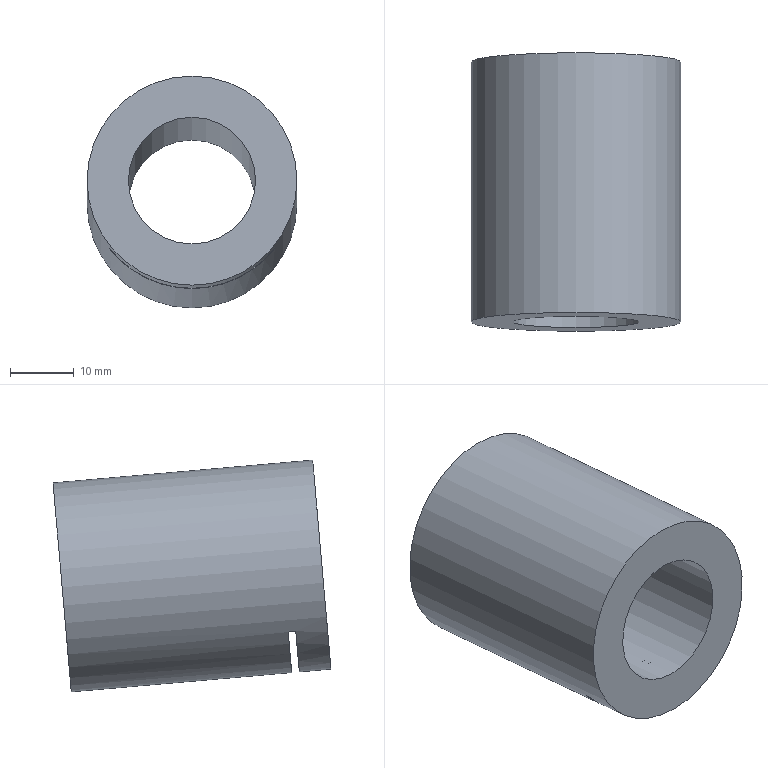Part | NX | features solid 2 | 1 solid | 7 faces | box 33 x 43.72 x 36.448 mm | volume 22047 mm3 | plane 5 | cylinder 2 | commonest cylinder face diameters 20 x1 33 x1
STEP:
#1=CARTESIAN_POINT('',(398.525,-75.036,-22.502));
#2=VERTEX_POINT('',#1);
#3=CARTESIAN_POINT('',(398.525,-76.474,-38.939));
#4=DIRECTION('',(0.,0.9962,-0.08716));
#5=DIRECTION('',(0.,0.08716,0.9962));
#6=AXIS2_PLACEMENT_3D('',#3,#4,#5);
#7=CIRCLE('',#6,16.5);
#8=EDGE_CURVE('',#2,#2,#7,.F.);
#9=ORIENTED_EDGE('',*,*,#8,.T.);
#10=EDGE_LOOP('',(#9));
#11=FACE_BOUND('',#10,.T.);
#12=CARTESIAN_POINT('',(398.525,-118.756,-51.803));
#13=VERTEX_POINT('',#12);
#14=CARTESIAN_POINT('',(398.525,-117.318,-35.366));
#15=DIRECTION('',(0.,-0.9962,0.08716));
#16=DIRECTION('',(0.,-0.08716,-0.9962));
#17=AXIS2_PLACEMENT_3D('',#14,#15,#16);
#18=CIRCLE('',#17,16.5);
#19=EDGE_CURVE('',#13,#13,#18,.T.);
#20=ORIENTED_EDGE('',*,*,#19,.F.);
#21=EDGE_LOOP('',(#20));
#22=FACE_BOUND('',#21,.T.);
#23=CARTESIAN_POINT('',(411.573,-113.217,-45.863));
#24=VERTEX_POINT('',#23);
#25=CARTESIAN_POINT('',(411.573,-112.021,-45.968));
#26=VERTEX_POINT('',#25);
#27=CARTESIAN_POINT('',(411.573,-76.358,-49.088));
#28=DIRECTION('',(0.,-0.9962,0.08716));
#29=VECTOR('',#28,1000.);
#30=LINE('',#27,#29);
#31=EDGE_CURVE('',#24,#26,#30,.F.);
#32=ORIENTED_EDGE('',*,*,#31,.T.);
#33=CARTESIAN_POINT('',(385.478,-112.021,-45.968));
#34=VERTEX_POINT('',#33);
#35=CARTESIAN_POINT('',(398.525,-111.141,-35.906));
#36=DIRECTION('',(0.,-0.9962,0.08716));
#37=DIRECTION('',(0.,-0.08716,-0.9962));
#38=AXIS2_PLACEMENT_3D('',#35,#36,#37);
#39=CIRCLE('',#38,16.5);
#40=EDGE_CURVE('',#26,#34,#39,.F.);
#41=ORIENTED_EDGE('',*,*,#40,.T.);
#42=CARTESIAN_POINT('',(385.478,-113.217,-45.863));
#43=VERTEX_POINT('',#42);
#44=CARTESIAN_POINT('',(385.478,-76.358,-49.088));
#45=DIRECTION('',(0.,-0.9962,0.08716));
#46=VECTOR('',#45,1000.);
#47=LINE('',#44,#46);
#48=EDGE_CURVE('',#34,#43,#47,.T.);
#49=ORIENTED_EDGE('',*,*,#48,.T.);
#50=CARTESIAN_POINT('',(398.525,-112.337,-35.802));
#51=DIRECTION('',(0.,-0.9962,0.08716));
#52=DIRECTION('',(0.,-0.08716,-0.9962));
#53=AXIS2_PLACEMENT_3D('',#50,#51,#52);
#54=CIRCLE('',#53,16.5);
#55=EDGE_CURVE('',#24,#43,#54,.F.);
#56=ORIENTED_EDGE('',*,*,#55,.F.);
#57=EDGE_LOOP('',(#32,#41,#49,#56));
#58=FACE_BOUND('',#57,.T.);
#59=CARTESIAN_POINT('',(398.525,-83.646,-38.312));
#60=DIRECTION('',(0.,-0.9962,0.08716));
#61=DIRECTION('',(0.,-0.08716,-0.9962));
#62=AXIS2_PLACEMENT_3D('',#59,#60,#61);
#63=CYLINDRICAL_SURFACE('',#62,16.5);
#64=ADVANCED_FACE('',(#11,#22,#58),#63,.T.);
#65=ORIENTED_EDGE('',*,*,#19,.T.);
#66=EDGE_LOOP('',(#65));
#67=FACE_BOUND('',#66,.T.);
#68=CARTESIAN_POINT('',(398.525,-118.189,-45.328));
#69=VERTEX_POINT('',#68);
#70=CARTESIAN_POINT('',(398.525,-117.318,-35.366));
#71=DIRECTION('',(0.,-0.9962,0.08716));
#72=DIRECTION('',(0.,-0.08716,-0.9962));
#73=AXIS2_PLACEMENT_3D('',#70,#71,#72);
#74=CIRCLE('',#73,10.);
#75=EDGE_CURVE('',#69,#69,#74,.T.);
#76=ORIENTED_EDGE('',*,*,#75,.F.);
#77=EDGE_LOOP('',(#76));
#78=FACE_BOUND('',#77,.T.);
#79=CARTESIAN_POINT('',(398.525,-117.318,-35.366));
#80=DIRECTION('',(0.,-0.9962,0.08716));
#81=DIRECTION('',(-1.,0.,0.));
#82=AXIS2_PLACEMENT_3D('',#79,#80,#81);
#83=PLANE('',#82);
#84=ADVANCED_FACE('',(#67,#78),#83,.T.);
#85=ORIENTED_EDGE('',*,*,#75,.T.);
#86=EDGE_LOOP('',(#85));
#87=FACE_BOUND('',#86,.T.);
#88=CARTESIAN_POINT('',(398.525,-75.602,-28.977));
#89=VERTEX_POINT('',#88);
#90=CARTESIAN_POINT('',(398.525,-76.474,-38.939));
#91=DIRECTION('',(0.,0.9962,-0.08716));
#92=DIRECTION('',(0.,0.08716,0.9962));
#93=AXIS2_PLACEMENT_3D('',#90,#91,#92);
#94=CIRCLE('',#93,10.);
#95=EDGE_CURVE('',#89,#89,#94,.F.);
#96=ORIENTED_EDGE('',*,*,#95,.F.);
#97=EDGE_LOOP('',(#96));
#98=FACE_BOUND('',#97,.T.);
#99=CARTESIAN_POINT('',(398.525,-69.699,-39.532));
#100=DIRECTION('',(0.,-0.9962,0.08716));
#101=DIRECTION('',(0.,-0.08716,-0.9962));
#102=AXIS2_PLACEMENT_3D('',#99,#100,#101);
#103=CYLINDRICAL_SURFACE('',#102,10.);
#104=ADVANCED_FACE('',(#87,#98),#103,.F.);
#105=ORIENTED_EDGE('',*,*,#8,.F.);
#106=EDGE_LOOP('',(#105));
#107=FACE_BOUND('',#106,.T.);
#108=ORIENTED_EDGE('',*,*,#95,.T.);
#109=EDGE_LOOP('',(#108));
#110=FACE_BOUND('',#109,.T.);
#111=CARTESIAN_POINT('',(398.525,-76.474,-38.939));
#112=DIRECTION('',(0.,0.9962,-0.08716));
#113=DIRECTION('',(-1.,0.,0.));
#114=AXIS2_PLACEMENT_3D('',#111,#112,#113);
#115=PLANE('',#114);
#116=ADVANCED_FACE('',(#107,#110),#115,.T.);
#117=CARTESIAN_POINT('',(385.401,-112.021,-45.968));
#118=DIRECTION('',(-1.,0.,0.));
#119=VECTOR('',#118,1000.);
#120=LINE('',#117,#119);
#121=EDGE_CURVE('',#34,#26,#120,.F.);
#122=ORIENTED_EDGE('',*,*,#121,.F.);
#123=ORIENTED_EDGE('',*,*,#40,.F.);
#124=EDGE_LOOP('',(#122,#123));
#125=FACE_BOUND('',#124,.T.);
#126=CARTESIAN_POINT('',(385.401,-116.379,-95.778));
#127=DIRECTION('',(0.,-0.9962,0.08716));
#128=DIRECTION('',(0.,-0.08716,-0.9962));
#129=AXIS2_PLACEMENT_3D('',#126,#127,#128);
#130=PLANE('',#129);
#131=ADVANCED_FACE('',(#125),#130,.T.);
#132=ORIENTED_EDGE('',*,*,#55,.T.);
#133=CARTESIAN_POINT('',(385.401,-113.217,-45.863));
#134=DIRECTION('',(-1.,0.,0.));
#135=VECTOR('',#134,1000.);
#136=LINE('',#133,#135);
#137=EDGE_CURVE('',#43,#24,#136,.F.);
#138=ORIENTED_EDGE('',*,*,#137,.T.);
#139=EDGE_LOOP('',(#132,#138));
#140=FACE_BOUND('',#139,.T.);
#141=CARTESIAN_POINT('',(385.401,-117.575,-95.673));
#142=DIRECTION('',(0.,-0.9962,0.08716));
#143=DIRECTION('',(0.,-0.08716,-0.9962));
#144=AXIS2_PLACEMENT_3D('',#141,#142,#143);
#145=PLANE('',#144);
#146=ADVANCED_FACE('',(#140),#145,.F.);
#147=ORIENTED_EDGE('',*,*,#121,.T.);
#148=ORIENTED_EDGE('',*,*,#31,.F.);
#149=ORIENTED_EDGE('',*,*,#137,.F.);
#150=ORIENTED_EDGE('',*,*,#48,.F.);
#151=EDGE_LOOP('',(#147,#148,#149,#150));
#152=FACE_BOUND('',#151,.T.);
#153=CARTESIAN_POINT('',(385.401,-113.217,-45.863));
#154=DIRECTION('',(0.,0.08716,0.9962));
#155=DIRECTION('',(0.,0.9962,-0.08716));
#156=AXIS2_PLACEMENT_3D('',#153,#154,#155);
#157=PLANE('',#156);
#158=ADVANCED_FACE('',(#152),#157,.F.);
#159=CLOSED_SHELL('',(#64,#84,#104,#116,#131,#146,#158));
#160=MANIFOLD_SOLID_BREP('',#159);
#161=(LENGTH_UNIT()NAMED_UNIT(*)SI_UNIT(.MILLI.,.METRE.));
#162=UNCERTAINTY_MEASURE_WITH_UNIT(LENGTH_MEASURE(0.00001),#161,'','');
#163=(NAMED_UNIT(*)PLANE_ANGLE_UNIT()SI_UNIT($,.RADIAN.));
#164=(NAMED_UNIT(*)SI_UNIT($,.STERADIAN.)SOLID_ANGLE_UNIT());
#165=(GEOMETRIC_REPRESENTATION_CONTEXT(3)GLOBAL_UNCERTAINTY_ASSIGNED_CONTEXT((#162))GLOBAL_UNIT_ASSIGNED_CONTEXT((#161,#163,#164))REPRESENTATION_CONTEXT('',''));
#166=ADVANCED_BREP_SHAPE_REPRESENTATION('',(#160),#165);